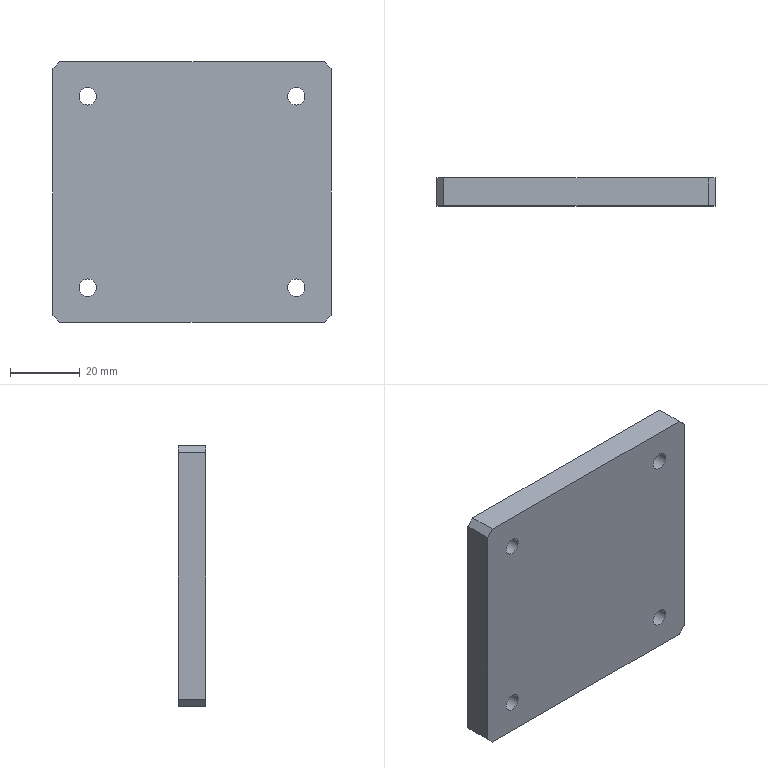Part | NX | 1 solid | 14 faces | box 80 x 8 x 75 mm | volume 47308 mm3 | plane 10 | cylinder 4 | commonest cylinder face diameters 5 x4
STEP:
#1=CARTESIAN_POINT('',(40.,8.,35.5));
#2=VERTEX_POINT('',#1);
#3=CARTESIAN_POINT('',(40.,8.,-35.5));
#4=VERTEX_POINT('',#3);
#5=CARTESIAN_POINT('',(40.,8.,37.5));
#6=DIRECTION('',(0.,0.,-1.));
#7=VECTOR('',#6,1000.);
#8=LINE('',#5,#7);
#9=EDGE_CURVE('',#2,#4,#8,.T.);
#10=ORIENTED_EDGE('',*,*,#9,.F.);
#11=CARTESIAN_POINT('',(40.,0.,35.5));
#12=VERTEX_POINT('',#11);
#13=CARTESIAN_POINT('',(40.,8.,35.5));
#14=DIRECTION('',(0.,-1.,0.));
#15=VECTOR('',#14,1000.);
#16=LINE('',#13,#15);
#17=EDGE_CURVE('',#2,#12,#16,.T.);
#18=ORIENTED_EDGE('',*,*,#17,.T.);
#19=CARTESIAN_POINT('',(40.,0.,-35.5));
#20=VERTEX_POINT('',#19);
#21=CARTESIAN_POINT('',(40.,0.,37.5));
#22=DIRECTION('',(0.,0.,-1.));
#23=VECTOR('',#22,1000.);
#24=LINE('',#21,#23);
#25=EDGE_CURVE('',#12,#20,#24,.T.);
#26=ORIENTED_EDGE('',*,*,#25,.T.);
#27=CARTESIAN_POINT('',(40.,8.,-35.5));
#28=DIRECTION('',(0.,1.,0.));
#29=VECTOR('',#28,1000.);
#30=LINE('',#27,#29);
#31=EDGE_CURVE('',#20,#4,#30,.T.);
#32=ORIENTED_EDGE('',*,*,#31,.T.);
#33=EDGE_LOOP('',(#10,#18,#26,#32));
#34=FACE_BOUND('',#33,.T.);
#35=CARTESIAN_POINT('',(40.,8.,37.5));
#36=DIRECTION('',(-1.,0.,0.));
#37=DIRECTION('',(0.,0.,1.));
#38=AXIS2_PLACEMENT_3D('',#35,#36,#37);
#39=PLANE('',#38);
#40=ADVANCED_FACE('',(#34),#39,.F.);
#41=CARTESIAN_POINT('',(38.,8.,-37.5));
#42=VERTEX_POINT('',#41);
#43=CARTESIAN_POINT('',(-38.,8.,-37.5));
#44=VERTEX_POINT('',#43);
#45=CARTESIAN_POINT('',(-40.,8.,-37.5));
#46=DIRECTION('',(-1.,0.,0.));
#47=VECTOR('',#46,1000.);
#48=LINE('',#45,#47);
#49=EDGE_CURVE('',#42,#44,#48,.T.);
#50=ORIENTED_EDGE('',*,*,#49,.F.);
#51=CARTESIAN_POINT('',(38.,0.,-37.5));
#52=VERTEX_POINT('',#51);
#53=CARTESIAN_POINT('',(38.,8.,-37.5));
#54=DIRECTION('',(0.,-1.,0.));
#55=VECTOR('',#54,1000.);
#56=LINE('',#53,#55);
#57=EDGE_CURVE('',#42,#52,#56,.T.);
#58=ORIENTED_EDGE('',*,*,#57,.T.);
#59=CARTESIAN_POINT('',(-38.,0.,-37.5));
#60=VERTEX_POINT('',#59);
#61=CARTESIAN_POINT('',(-40.,0.,-37.5));
#62=DIRECTION('',(-1.,0.,0.));
#63=VECTOR('',#62,1000.);
#64=LINE('',#61,#63);
#65=EDGE_CURVE('',#52,#60,#64,.T.);
#66=ORIENTED_EDGE('',*,*,#65,.T.);
#67=CARTESIAN_POINT('',(-38.,8.,-37.5));
#68=DIRECTION('',(0.,1.,0.));
#69=VECTOR('',#68,1000.);
#70=LINE('',#67,#69);
#71=EDGE_CURVE('',#60,#44,#70,.T.);
#72=ORIENTED_EDGE('',*,*,#71,.T.);
#73=EDGE_LOOP('',(#50,#58,#66,#72));
#74=FACE_BOUND('',#73,.T.);
#75=CARTESIAN_POINT('',(-40.,8.,-37.5));
#76=DIRECTION('',(0.,0.,1.));
#77=DIRECTION('',(1.,0.,0.));
#78=AXIS2_PLACEMENT_3D('',#75,#76,#77);
#79=PLANE('',#78);
#80=ADVANCED_FACE('',(#74),#79,.F.);
#81=CARTESIAN_POINT('',(-40.,0.,-35.5));
#82=VERTEX_POINT('',#81);
#83=CARTESIAN_POINT('',(-40.,0.,35.5));
#84=VERTEX_POINT('',#83);
#85=CARTESIAN_POINT('',(-40.,0.,37.5));
#86=DIRECTION('',(0.,0.,1.));
#87=VECTOR('',#86,1000.);
#88=LINE('',#85,#87);
#89=EDGE_CURVE('',#82,#84,#88,.T.);
#90=ORIENTED_EDGE('',*,*,#89,.T.);
#91=CARTESIAN_POINT('',(-40.,8.,35.5));
#92=VERTEX_POINT('',#91);
#93=CARTESIAN_POINT('',(-40.,8.,35.5));
#94=DIRECTION('',(0.,1.,0.));
#95=VECTOR('',#94,1000.);
#96=LINE('',#93,#95);
#97=EDGE_CURVE('',#84,#92,#96,.T.);
#98=ORIENTED_EDGE('',*,*,#97,.T.);
#99=CARTESIAN_POINT('',(-40.,8.,-35.5));
#100=VERTEX_POINT('',#99);
#101=CARTESIAN_POINT('',(-40.,8.,37.5));
#102=DIRECTION('',(0.,0.,1.));
#103=VECTOR('',#102,1000.);
#104=LINE('',#101,#103);
#105=EDGE_CURVE('',#100,#92,#104,.T.);
#106=ORIENTED_EDGE('',*,*,#105,.F.);
#107=CARTESIAN_POINT('',(-40.,8.,-35.5));
#108=DIRECTION('',(0.,-1.,0.));
#109=VECTOR('',#108,1000.);
#110=LINE('',#107,#109);
#111=EDGE_CURVE('',#100,#82,#110,.T.);
#112=ORIENTED_EDGE('',*,*,#111,.T.);
#113=EDGE_LOOP('',(#90,#98,#106,#112));
#114=FACE_BOUND('',#113,.T.);
#115=CARTESIAN_POINT('',(-40.,8.,37.5));
#116=DIRECTION('',(1.,0.,0.));
#117=DIRECTION('',(0.,0.,-1.));
#118=AXIS2_PLACEMENT_3D('',#115,#116,#117);
#119=PLANE('',#118);
#120=ADVANCED_FACE('',(#114),#119,.F.);
#121=CARTESIAN_POINT('',(-38.,8.,37.5));
#122=VERTEX_POINT('',#121);
#123=CARTESIAN_POINT('',(38.,8.,37.5));
#124=VERTEX_POINT('',#123);
#125=CARTESIAN_POINT('',(-40.,8.,37.5));
#126=DIRECTION('',(1.,0.,0.));
#127=VECTOR('',#126,1000.);
#128=LINE('',#125,#127);
#129=EDGE_CURVE('',#122,#124,#128,.T.);
#130=ORIENTED_EDGE('',*,*,#129,.F.);
#131=CARTESIAN_POINT('',(-38.,0.,37.5));
#132=VERTEX_POINT('',#131);
#133=CARTESIAN_POINT('',(-38.,8.,37.5));
#134=DIRECTION('',(0.,-1.,0.));
#135=VECTOR('',#134,1000.);
#136=LINE('',#133,#135);
#137=EDGE_CURVE('',#122,#132,#136,.T.);
#138=ORIENTED_EDGE('',*,*,#137,.T.);
#139=CARTESIAN_POINT('',(38.,0.,37.5));
#140=VERTEX_POINT('',#139);
#141=CARTESIAN_POINT('',(-40.,0.,37.5));
#142=DIRECTION('',(1.,0.,0.));
#143=VECTOR('',#142,1000.);
#144=LINE('',#141,#143);
#145=EDGE_CURVE('',#132,#140,#144,.T.);
#146=ORIENTED_EDGE('',*,*,#145,.T.);
#147=CARTESIAN_POINT('',(38.,8.,37.5));
#148=DIRECTION('',(0.,1.,0.));
#149=VECTOR('',#148,1000.);
#150=LINE('',#147,#149);
#151=EDGE_CURVE('',#140,#124,#150,.T.);
#152=ORIENTED_EDGE('',*,*,#151,.T.);
#153=EDGE_LOOP('',(#130,#138,#146,#152));
#154=FACE_BOUND('',#153,.T.);
#155=CARTESIAN_POINT('',(-40.,8.,37.5));
#156=DIRECTION('',(0.,0.,-1.));
#157=DIRECTION('',(-1.,0.,0.));
#158=AXIS2_PLACEMENT_3D('',#155,#156,#157);
#159=PLANE('',#158);
#160=ADVANCED_FACE('',(#154),#159,.F.);
#161=CARTESIAN_POINT('',(-30.,8.,-25.));
#162=VERTEX_POINT('',#161);
#163=CARTESIAN_POINT('',(-30.,8.,-27.5));
#164=DIRECTION('',(0.,1.,0.));
#165=DIRECTION('',(0.,0.,1.));
#166=AXIS2_PLACEMENT_3D('',#163,#164,#165);
#167=CIRCLE('',#166,2.5);
#168=EDGE_CURVE('',#162,#162,#167,.T.);
#169=ORIENTED_EDGE('',*,*,#168,.F.);
#170=EDGE_LOOP('',(#169));
#171=FACE_BOUND('',#170,.T.);
#172=CARTESIAN_POINT('',(30.,8.,-25.));
#173=VERTEX_POINT('',#172);
#174=CARTESIAN_POINT('',(30.,8.,-27.5));
#175=DIRECTION('',(0.,1.,0.));
#176=DIRECTION('',(0.,0.,1.));
#177=AXIS2_PLACEMENT_3D('',#174,#175,#176);
#178=CIRCLE('',#177,2.5);
#179=EDGE_CURVE('',#173,#173,#178,.T.);
#180=ORIENTED_EDGE('',*,*,#179,.F.);
#181=EDGE_LOOP('',(#180));
#182=FACE_BOUND('',#181,.T.);
#183=CARTESIAN_POINT('',(30.,8.,30.));
#184=VERTEX_POINT('',#183);
#185=CARTESIAN_POINT('',(30.,8.,27.5));
#186=DIRECTION('',(0.,1.,0.));
#187=DIRECTION('',(0.,0.,1.));
#188=AXIS2_PLACEMENT_3D('',#185,#186,#187);
#189=CIRCLE('',#188,2.5);
#190=EDGE_CURVE('',#184,#184,#189,.T.);
#191=ORIENTED_EDGE('',*,*,#190,.F.);
#192=EDGE_LOOP('',(#191));
#193=FACE_BOUND('',#192,.T.);
#194=CARTESIAN_POINT('',(-30.,8.,30.));
#195=VERTEX_POINT('',#194);
#196=CARTESIAN_POINT('',(-30.,8.,27.5));
#197=DIRECTION('',(0.,1.,0.));
#198=DIRECTION('',(0.,0.,1.));
#199=AXIS2_PLACEMENT_3D('',#196,#197,#198);
#200=CIRCLE('',#199,2.5);
#201=EDGE_CURVE('',#195,#195,#200,.T.);
#202=ORIENTED_EDGE('',*,*,#201,.F.);
#203=EDGE_LOOP('',(#202));
#204=FACE_BOUND('',#203,.T.);
#205=ORIENTED_EDGE('',*,*,#105,.T.);
#206=CARTESIAN_POINT('',(-38.,8.,37.5));
#207=DIRECTION('',(-0.7071,0.,-0.7071));
#208=VECTOR('',#207,1000.);
#209=LINE('',#206,#208);
#210=EDGE_CURVE('',#92,#122,#209,.F.);
#211=ORIENTED_EDGE('',*,*,#210,.T.);
#212=ORIENTED_EDGE('',*,*,#129,.T.);
#213=CARTESIAN_POINT('',(40.,8.,35.5));
#214=DIRECTION('',(-0.7071,0.,0.7071));
#215=VECTOR('',#214,1000.);
#216=LINE('',#213,#215);
#217=EDGE_CURVE('',#124,#2,#216,.F.);
#218=ORIENTED_EDGE('',*,*,#217,.T.);
#219=ORIENTED_EDGE('',*,*,#9,.T.);
#220=CARTESIAN_POINT('',(38.,8.,-37.5));
#221=DIRECTION('',(0.7071,0.,0.7071));
#222=VECTOR('',#221,1000.);
#223=LINE('',#220,#222);
#224=EDGE_CURVE('',#4,#42,#223,.F.);
#225=ORIENTED_EDGE('',*,*,#224,.T.);
#226=ORIENTED_EDGE('',*,*,#49,.T.);
#227=CARTESIAN_POINT('',(-40.,8.,-35.5));
#228=DIRECTION('',(0.7071,0.,-0.7071));
#229=VECTOR('',#228,1000.);
#230=LINE('',#227,#229);
#231=EDGE_CURVE('',#44,#100,#230,.F.);
#232=ORIENTED_EDGE('',*,*,#231,.T.);
#233=EDGE_LOOP('',(#205,#211,#212,#218,#219,#225,#226,#232));
#234=FACE_BOUND('',#233,.T.);
#235=CARTESIAN_POINT('',(0.,8.,0.));
#236=DIRECTION('',(0.,-1.,0.));
#237=DIRECTION('',(0.,0.,-1.));
#238=AXIS2_PLACEMENT_3D('',#235,#236,#237);
#239=PLANE('',#238);
#240=ADVANCED_FACE('',(#171,#182,#193,#204,#234),#239,.F.);
#241=CARTESIAN_POINT('',(-30.,0.,-25.));
#242=VERTEX_POINT('',#241);
#243=CARTESIAN_POINT('',(-30.,0.,-27.5));
#244=DIRECTION('',(0.,1.,0.));
#245=DIRECTION('',(0.,0.,1.));
#246=AXIS2_PLACEMENT_3D('',#243,#244,#245);
#247=CIRCLE('',#246,2.5);
#248=EDGE_CURVE('',#242,#242,#247,.T.);
#249=ORIENTED_EDGE('',*,*,#248,.T.);
#250=EDGE_LOOP('',(#249));
#251=FACE_BOUND('',#250,.T.);
#252=CARTESIAN_POINT('',(30.,0.,-25.));
#253=VERTEX_POINT('',#252);
#254=CARTESIAN_POINT('',(30.,0.,-27.5));
#255=DIRECTION('',(0.,1.,0.));
#256=DIRECTION('',(0.,0.,1.));
#257=AXIS2_PLACEMENT_3D('',#254,#255,#256);
#258=CIRCLE('',#257,2.5);
#259=EDGE_CURVE('',#253,#253,#258,.T.);
#260=ORIENTED_EDGE('',*,*,#259,.T.);
#261=EDGE_LOOP('',(#260));
#262=FACE_BOUND('',#261,.T.);
#263=CARTESIAN_POINT('',(30.,0.,30.));
#264=VERTEX_POINT('',#263);
#265=CARTESIAN_POINT('',(30.,0.,27.5));
#266=DIRECTION('',(0.,1.,0.));
#267=DIRECTION('',(0.,0.,1.));
#268=AXIS2_PLACEMENT_3D('',#265,#266,#267);
#269=CIRCLE('',#268,2.5);
#270=EDGE_CURVE('',#264,#264,#269,.T.);
#271=ORIENTED_EDGE('',*,*,#270,.T.);
#272=EDGE_LOOP('',(#271));
#273=FACE_BOUND('',#272,.T.);
#274=CARTESIAN_POINT('',(-30.,0.,30.));
#275=VERTEX_POINT('',#274);
#276=CARTESIAN_POINT('',(-30.,0.,27.5));
#277=DIRECTION('',(0.,1.,0.));
#278=DIRECTION('',(0.,0.,1.));
#279=AXIS2_PLACEMENT_3D('',#276,#277,#278);
#280=CIRCLE('',#279,2.5);
#281=EDGE_CURVE('',#275,#275,#280,.T.);
#282=ORIENTED_EDGE('',*,*,#281,.T.);
#283=EDGE_LOOP('',(#282));
#284=FACE_BOUND('',#283,.T.);
#285=ORIENTED_EDGE('',*,*,#145,.F.);
#286=CARTESIAN_POINT('',(-37.75,0.,37.75));
#287=DIRECTION('',(0.7071,0.,0.7071));
#288=VECTOR('',#287,1000.);
#289=LINE('',#286,#288);
#290=EDGE_CURVE('',#132,#84,#289,.F.);
#291=ORIENTED_EDGE('',*,*,#290,.T.);
#292=ORIENTED_EDGE('',*,*,#89,.F.);
#293=CARTESIAN_POINT('',(-37.75,0.,-37.75));
#294=DIRECTION('',(-0.7071,0.,0.7071));
#295=VECTOR('',#294,1000.);
#296=LINE('',#293,#295);
#297=EDGE_CURVE('',#82,#60,#296,.F.);
#298=ORIENTED_EDGE('',*,*,#297,.T.);
#299=ORIENTED_EDGE('',*,*,#65,.F.);
#300=CARTESIAN_POINT('',(37.75,0.,-37.75));
#301=DIRECTION('',(-0.7071,0.,-0.7071));
#302=VECTOR('',#301,1000.);
#303=LINE('',#300,#302);
#304=EDGE_CURVE('',#52,#20,#303,.F.);
#305=ORIENTED_EDGE('',*,*,#304,.T.);
#306=ORIENTED_EDGE('',*,*,#25,.F.);
#307=CARTESIAN_POINT('',(37.75,0.,37.75));
#308=DIRECTION('',(0.7071,0.,-0.7071));
#309=VECTOR('',#308,1000.);
#310=LINE('',#307,#309);
#311=EDGE_CURVE('',#12,#140,#310,.F.);
#312=ORIENTED_EDGE('',*,*,#311,.T.);
#313=EDGE_LOOP('',(#285,#291,#292,#298,#299,#305,#306,#312));
#314=FACE_BOUND('',#313,.T.);
#315=CARTESIAN_POINT('',(0.,0.,0.));
#316=DIRECTION('',(0.,-1.,0.));
#317=DIRECTION('',(0.,0.,-1.));
#318=AXIS2_PLACEMENT_3D('',#315,#316,#317);
#319=PLANE('',#318);
#320=ADVANCED_FACE('',(#251,#262,#273,#284,#314),#319,.T.);
#321=ORIENTED_EDGE('',*,*,#210,.F.);
#322=ORIENTED_EDGE('',*,*,#97,.F.);
#323=ORIENTED_EDGE('',*,*,#290,.F.);
#324=ORIENTED_EDGE('',*,*,#137,.F.);
#325=EDGE_LOOP('',(#321,#322,#323,#324));
#326=FACE_BOUND('',#325,.T.);
#327=CARTESIAN_POINT('',(-38.,8.,37.5));
#328=DIRECTION('',(0.7071,0.,-0.7071));
#329=DIRECTION('',(0.,-1.,0.));
#330=AXIS2_PLACEMENT_3D('',#327,#328,#329);
#331=PLANE('',#330);
#332=ADVANCED_FACE('',(#326),#331,.F.);
#333=ORIENTED_EDGE('',*,*,#217,.F.);
#334=ORIENTED_EDGE('',*,*,#151,.F.);
#335=ORIENTED_EDGE('',*,*,#311,.F.);
#336=ORIENTED_EDGE('',*,*,#17,.F.);
#337=EDGE_LOOP('',(#333,#334,#335,#336));
#338=FACE_BOUND('',#337,.T.);
#339=CARTESIAN_POINT('',(40.,8.,35.5));
#340=DIRECTION('',(-0.7071,0.,-0.7071));
#341=DIRECTION('',(0.,-1.,0.));
#342=AXIS2_PLACEMENT_3D('',#339,#340,#341);
#343=PLANE('',#342);
#344=ADVANCED_FACE('',(#338),#343,.F.);
#345=ORIENTED_EDGE('',*,*,#224,.F.);
#346=ORIENTED_EDGE('',*,*,#31,.F.);
#347=ORIENTED_EDGE('',*,*,#304,.F.);
#348=ORIENTED_EDGE('',*,*,#57,.F.);
#349=EDGE_LOOP('',(#345,#346,#347,#348));
#350=FACE_BOUND('',#349,.T.);
#351=CARTESIAN_POINT('',(38.,8.,-37.5));
#352=DIRECTION('',(-0.7071,0.,0.7071));
#353=DIRECTION('',(0.,-1.,0.));
#354=AXIS2_PLACEMENT_3D('',#351,#352,#353);
#355=PLANE('',#354);
#356=ADVANCED_FACE('',(#350),#355,.F.);
#357=ORIENTED_EDGE('',*,*,#231,.F.);
#358=ORIENTED_EDGE('',*,*,#71,.F.);
#359=ORIENTED_EDGE('',*,*,#297,.F.);
#360=ORIENTED_EDGE('',*,*,#111,.F.);
#361=EDGE_LOOP('',(#357,#358,#359,#360));
#362=FACE_BOUND('',#361,.T.);
#363=CARTESIAN_POINT('',(-40.,8.,-35.5));
#364=DIRECTION('',(0.7071,0.,0.7071));
#365=DIRECTION('',(0.,-1.,0.));
#366=AXIS2_PLACEMENT_3D('',#363,#364,#365);
#367=PLANE('',#366);
#368=ADVANCED_FACE('',(#362),#367,.F.);
#369=ORIENTED_EDGE('',*,*,#281,.F.);
#370=EDGE_LOOP('',(#369));
#371=FACE_BOUND('',#370,.T.);
#372=ORIENTED_EDGE('',*,*,#201,.T.);
#373=EDGE_LOOP('',(#372));
#374=FACE_BOUND('',#373,.T.);
#375=CARTESIAN_POINT('',(-30.,8.,27.5));
#376=DIRECTION('',(0.,1.,0.));
#377=DIRECTION('',(0.,0.,1.));
#378=AXIS2_PLACEMENT_3D('',#375,#376,#377);
#379=CYLINDRICAL_SURFACE('',#378,2.5);
#380=ADVANCED_FACE('',(#371,#374),#379,.F.);
#381=ORIENTED_EDGE('',*,*,#270,.F.);
#382=EDGE_LOOP('',(#381));
#383=FACE_BOUND('',#382,.T.);
#384=ORIENTED_EDGE('',*,*,#190,.T.);
#385=EDGE_LOOP('',(#384));
#386=FACE_BOUND('',#385,.T.);
#387=CARTESIAN_POINT('',(30.,8.,27.5));
#388=DIRECTION('',(0.,1.,0.));
#389=DIRECTION('',(0.,0.,1.));
#390=AXIS2_PLACEMENT_3D('',#387,#388,#389);
#391=CYLINDRICAL_SURFACE('',#390,2.5);
#392=ADVANCED_FACE('',(#383,#386),#391,.F.);
#393=ORIENTED_EDGE('',*,*,#259,.F.);
#394=EDGE_LOOP('',(#393));
#395=FACE_BOUND('',#394,.T.);
#396=ORIENTED_EDGE('',*,*,#179,.T.);
#397=EDGE_LOOP('',(#396));
#398=FACE_BOUND('',#397,.T.);
#399=CARTESIAN_POINT('',(30.,8.,-27.5));
#400=DIRECTION('',(0.,1.,0.));
#401=DIRECTION('',(0.,0.,1.));
#402=AXIS2_PLACEMENT_3D('',#399,#400,#401);
#403=CYLINDRICAL_SURFACE('',#402,2.5);
#404=ADVANCED_FACE('',(#395,#398),#403,.F.);
#405=ORIENTED_EDGE('',*,*,#248,.F.);
#406=EDGE_LOOP('',(#405));
#407=FACE_BOUND('',#406,.T.);
#408=ORIENTED_EDGE('',*,*,#168,.T.);
#409=EDGE_LOOP('',(#408));
#410=FACE_BOUND('',#409,.T.);
#411=CARTESIAN_POINT('',(-30.,8.,-27.5));
#412=DIRECTION('',(0.,1.,0.));
#413=DIRECTION('',(0.,0.,1.));
#414=AXIS2_PLACEMENT_3D('',#411,#412,#413);
#415=CYLINDRICAL_SURFACE('',#414,2.5);
#416=ADVANCED_FACE('',(#407,#410),#415,.F.);
#417=CLOSED_SHELL('',(#40,#80,#120,#160,#240,#320,#332,#344,#356,#368,#380,#392,#404,#416));
#418=MANIFOLD_SOLID_BREP('',#417);
#419=(LENGTH_UNIT()NAMED_UNIT(*)SI_UNIT(.MILLI.,.METRE.));
#420=UNCERTAINTY_MEASURE_WITH_UNIT(LENGTH_MEASURE(0.00001),#419,'','');
#421=(NAMED_UNIT(*)PLANE_ANGLE_UNIT()SI_UNIT($,.RADIAN.));
#422=(NAMED_UNIT(*)SI_UNIT($,.STERADIAN.)SOLID_ANGLE_UNIT());
#423=(GEOMETRIC_REPRESENTATION_CONTEXT(3)GLOBAL_UNCERTAINTY_ASSIGNED_CONTEXT((#420))GLOBAL_UNIT_ASSIGNED_CONTEXT((#419,#421,#422))REPRESENTATION_CONTEXT('',''));
#424=ADVANCED_BREP_SHAPE_REPRESENTATION('',(#418),#423);